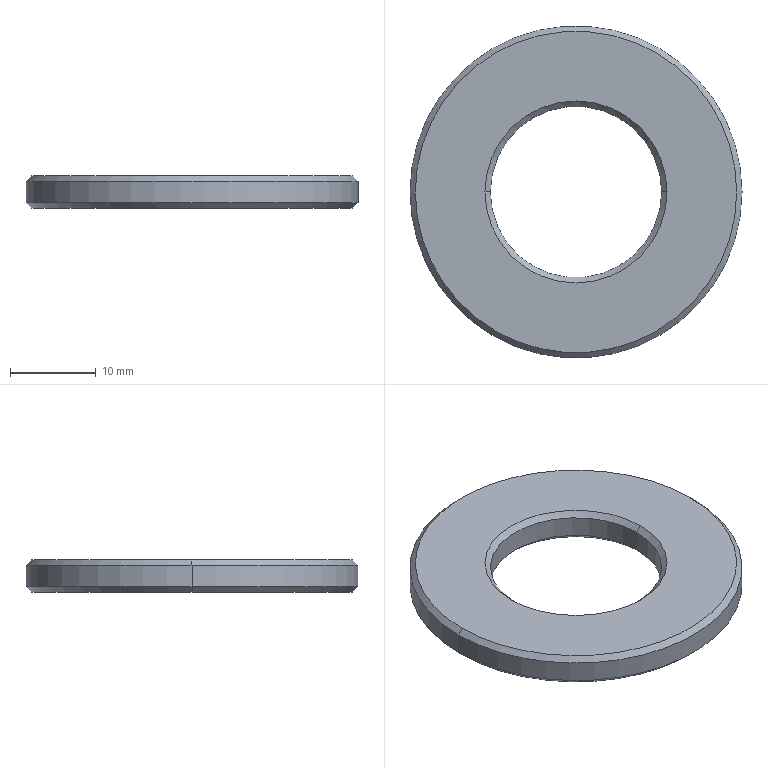Part | Creo | features DATUM PLANE 3, CHAMFER 1, COORDINATE SYSTEM 1, CURVE 1, PROTRUSION 1 | 1 solid | 14 faces | box 38.75 x 38.75 x 3.75 mm | volume 3172 mm3 | cone 8 | cylinder 4 | plane 2 | commonest cylinder face diameters 20 x2 38.75 x2
STEP:
#1=CARTESIAN_POINT('',(0.,0.,0.));
#2=DIRECTION('',(0.,0.,1.));
#3=DIRECTION('',(1.,0.,0.));
#4=AXIS2_PLACEMENT_3D('',#1,#2,#3);
#5=CARTESIAN_POINT('',(-18.75,0.,0.));
#6=VERTEX_POINT('',#5);
#7=CARTESIAN_POINT('',(18.75,0.,0.));
#8=VERTEX_POINT('',#7);
#9=CARTESIAN_POINT('',(0.,0.,0.));
#10=DIRECTION('',(0.,0.,-1.));
#11=DIRECTION('',(-1.,0.,0.));
#12=AXIS2_PLACEMENT_3D('',#9,#10,#11);
#13=CIRCLE('',#12,18.75);
#14=EDGE_CURVE('',#6,#8,#13,.T.);
#15=ORIENTED_EDGE('',*,*,#14,.F.);
#16=CARTESIAN_POINT('',(0.,0.,0.));
#17=DIRECTION('',(0.,0.,-1.));
#18=DIRECTION('',(1.,0.,0.));
#19=AXIS2_PLACEMENT_3D('',#16,#17,#18);
#20=CIRCLE('',#19,18.75);
#21=EDGE_CURVE('',#8,#6,#20,.T.);
#22=ORIENTED_EDGE('',*,*,#21,.F.);
#23=EDGE_LOOP('',(#15,#22));
#24=FACE_OUTER_BOUND('',#23,.F.);
#25=CARTESIAN_POINT('',(-10.625,0.,0.));
#26=VERTEX_POINT('',#25);
#27=CARTESIAN_POINT('',(10.625,0.,0.));
#28=VERTEX_POINT('',#27);
#29=CARTESIAN_POINT('',(0.,0.,0.));
#30=DIRECTION('',(0.,0.,1.));
#31=DIRECTION('',(-1.,0.,0.));
#32=AXIS2_PLACEMENT_3D('',#29,#30,#31);
#33=CIRCLE('',#32,10.625);
#34=EDGE_CURVE('',#26,#28,#33,.T.);
#35=ORIENTED_EDGE('',*,*,#34,.F.);
#36=CARTESIAN_POINT('',(0.,0.,0.));
#37=DIRECTION('',(0.,0.,1.));
#38=DIRECTION('',(1.,0.,0.));
#39=AXIS2_PLACEMENT_3D('',#36,#37,#38);
#40=CIRCLE('',#39,10.625);
#41=EDGE_CURVE('',#28,#26,#40,.T.);
#42=ORIENTED_EDGE('',*,*,#41,.F.);
#43=EDGE_LOOP('',(#35,#42));
#44=FACE_BOUND('',#43,.F.);
#45=CARTESIAN_POINT('',(0.,0.,0.));
#46=DIRECTION('',(0.,0.,1.));
#47=DIRECTION('',(1.,0.,0.));
#48=AXIS2_PLACEMENT_3D('',#45,#46,#47);
#49=PLANE('',#48);
#50=ADVANCED_FACE('',(#24,#44),#49,.F.);
#51=ORIENTED_EDGE('',*,*,#14,.T.);
#52=CARTESIAN_POINT('',(19.375,0.,0.625));
#53=VERTEX_POINT('',#52);
#54=CARTESIAN_POINT('',(18.75,0.000000003,0.));
#55=DIRECTION('',(0.7071,-0.000000001,0.7071));
#56=VECTOR('',#55,0.8839);
#57=LINE('',#54,#56);
#58=EDGE_CURVE('',#8,#53,#57,.T.);
#59=ORIENTED_EDGE('',*,*,#58,.T.);
#60=CARTESIAN_POINT('',(-19.375,0.,0.625));
#61=VERTEX_POINT('',#60);
#62=CARTESIAN_POINT('',(0.,0.,0.625));
#63=DIRECTION('',(0.,0.,-1.));
#64=DIRECTION('',(-1.,0.,0.));
#65=AXIS2_PLACEMENT_3D('',#62,#63,#64);
#66=CIRCLE('',#65,19.375);
#67=EDGE_CURVE('',#61,#53,#66,.T.);
#68=ORIENTED_EDGE('',*,*,#67,.F.);
#69=CARTESIAN_POINT('',(-18.75,-0.000000003,0.));
#70=DIRECTION('',(-0.7071,0.000000001,0.7071));
#71=VECTOR('',#70,0.8839);
#72=LINE('',#69,#71);
#73=EDGE_CURVE('',#6,#61,#72,.T.);
#74=ORIENTED_EDGE('',*,*,#73,.F.);
#75=EDGE_LOOP('',(#51,#59,#68,#74));
#76=FACE_OUTER_BOUND('',#75,.F.);
#77=CARTESIAN_POINT('',(0.,0.,0.3125));
#78=DIRECTION('',(0.,0.,1.));
#79=DIRECTION('',(0.,-1.,0.));
#80=AXIS2_PLACEMENT_3D('',#77,#78,#79);
#81=CONICAL_SURFACE('',#80,19.062,45.);
#82=ADVANCED_FACE('',(#76),#81,.T.);
#83=ORIENTED_EDGE('',*,*,#21,.T.);
#84=ORIENTED_EDGE('',*,*,#73,.T.);
#85=CARTESIAN_POINT('',(0.,0.,0.625));
#86=DIRECTION('',(0.,0.,-1.));
#87=DIRECTION('',(1.,0.,0.));
#88=AXIS2_PLACEMENT_3D('',#85,#86,#87);
#89=CIRCLE('',#88,19.375);
#90=EDGE_CURVE('',#53,#61,#89,.T.);
#91=ORIENTED_EDGE('',*,*,#90,.F.);
#92=ORIENTED_EDGE('',*,*,#58,.F.);
#93=EDGE_LOOP('',(#83,#84,#91,#92));
#94=FACE_OUTER_BOUND('',#93,.F.);
#95=CARTESIAN_POINT('',(0.,0.,0.3125));
#96=DIRECTION('',(0.,0.,1.));
#97=DIRECTION('',(0.,-1.,0.));
#98=AXIS2_PLACEMENT_3D('',#95,#96,#97);
#99=CONICAL_SURFACE('',#98,19.062,45.);
#100=ADVANCED_FACE('',(#94),#99,.T.);
#101=CARTESIAN_POINT('',(-19.375,0.,3.125));
#102=VERTEX_POINT('',#101);
#103=CARTESIAN_POINT('',(19.375,0.,3.125));
#104=VERTEX_POINT('',#103);
#105=CARTESIAN_POINT('',(0.,0.,3.125));
#106=DIRECTION('',(0.,0.,1.));
#107=DIRECTION('',(-1.,0.,0.));
#108=AXIS2_PLACEMENT_3D('',#105,#106,#107);
#109=CIRCLE('',#108,19.375);
#110=EDGE_CURVE('',#102,#104,#109,.T.);
#111=ORIENTED_EDGE('',*,*,#110,.T.);
#112=CARTESIAN_POINT('',(19.375,0.000000002,0.625));
#113=DIRECTION('',(0.,0.,1.));
#114=VECTOR('',#113,2.5);
#115=LINE('',#112,#114);
#116=EDGE_CURVE('',#53,#104,#115,.T.);
#117=ORIENTED_EDGE('',*,*,#116,.F.);
#118=ORIENTED_EDGE('',*,*,#90,.T.);
#119=CARTESIAN_POINT('',(-19.375,-0.000000002,0.625));
#120=DIRECTION('',(0.,0.,1.));
#121=VECTOR('',#120,2.5);
#122=LINE('',#119,#121);
#123=EDGE_CURVE('',#61,#102,#122,.T.);
#124=ORIENTED_EDGE('',*,*,#123,.T.);
#125=EDGE_LOOP('',(#111,#117,#118,#124));
#126=FACE_OUTER_BOUND('',#125,.F.);
#127=CARTESIAN_POINT('',(0.,0.,0.));
#128=DIRECTION('',(0.,0.,1.));
#129=DIRECTION('',(1.,0.,0.));
#130=AXIS2_PLACEMENT_3D('',#127,#128,#129);
#131=CYLINDRICAL_SURFACE('',#130,19.375);
#132=ADVANCED_FACE('',(#126),#131,.T.);
#133=CARTESIAN_POINT('',(-18.75,0.,3.75));
#134=VERTEX_POINT('',#133);
#135=CARTESIAN_POINT('',(18.75,0.,3.75));
#136=VERTEX_POINT('',#135);
#137=CARTESIAN_POINT('',(0.,0.,3.75));
#138=DIRECTION('',(0.,0.,1.));
#139=DIRECTION('',(-1.,0.,0.));
#140=AXIS2_PLACEMENT_3D('',#137,#138,#139);
#141=CIRCLE('',#140,18.75);
#142=EDGE_CURVE('',#134,#136,#141,.T.);
#143=ORIENTED_EDGE('',*,*,#142,.T.);
#144=CARTESIAN_POINT('',(18.75,0.000000003,3.75));
#145=DIRECTION('',(0.7071,-0.000000001,-0.7071));
#146=VECTOR('',#145,0.8839);
#147=LINE('',#144,#146);
#148=EDGE_CURVE('',#136,#104,#147,.T.);
#149=ORIENTED_EDGE('',*,*,#148,.T.);
#150=ORIENTED_EDGE('',*,*,#110,.F.);
#151=CARTESIAN_POINT('',(-18.75,-0.000000003,3.75));
#152=DIRECTION('',(-0.7071,0.000000001,-0.7071));
#153=VECTOR('',#152,0.8839);
#154=LINE('',#151,#153);
#155=EDGE_CURVE('',#134,#102,#154,.T.);
#156=ORIENTED_EDGE('',*,*,#155,.F.);
#157=EDGE_LOOP('',(#143,#149,#150,#156));
#158=FACE_OUTER_BOUND('',#157,.F.);
#159=CARTESIAN_POINT('',(0.,0.,3.438));
#160=DIRECTION('',(0.,0.,-1.));
#161=DIRECTION('',(0.,-1.,0.));
#162=AXIS2_PLACEMENT_3D('',#159,#160,#161);
#163=CONICAL_SURFACE('',#162,19.062,45.);
#164=ADVANCED_FACE('',(#158),#163,.T.);
#165=CARTESIAN_POINT('',(0.,0.,3.75));
#166=DIRECTION('',(0.,0.,1.));
#167=DIRECTION('',(1.,0.,0.));
#168=AXIS2_PLACEMENT_3D('',#165,#166,#167);
#169=CIRCLE('',#168,18.75);
#170=EDGE_CURVE('',#136,#134,#169,.T.);
#171=ORIENTED_EDGE('',*,*,#170,.F.);
#172=ORIENTED_EDGE('',*,*,#142,.F.);
#173=EDGE_LOOP('',(#171,#172));
#174=FACE_OUTER_BOUND('',#173,.F.);
#175=CARTESIAN_POINT('',(10.625,0.,3.75));
#176=VERTEX_POINT('',#175);
#177=CARTESIAN_POINT('',(-10.625,0.,3.75));
#178=VERTEX_POINT('',#177);
#179=CARTESIAN_POINT('',(0.,0.,3.75));
#180=DIRECTION('',(0.,0.,-1.));
#181=DIRECTION('',(1.,0.,0.));
#182=AXIS2_PLACEMENT_3D('',#179,#180,#181);
#183=CIRCLE('',#182,10.625);
#184=EDGE_CURVE('',#176,#178,#183,.T.);
#185=ORIENTED_EDGE('',*,*,#184,.F.);
#186=CARTESIAN_POINT('',(0.,0.,3.75));
#187=DIRECTION('',(0.,0.,-1.));
#188=DIRECTION('',(-1.,0.,0.));
#189=AXIS2_PLACEMENT_3D('',#186,#187,#188);
#190=CIRCLE('',#189,10.625);
#191=EDGE_CURVE('',#178,#176,#190,.T.);
#192=ORIENTED_EDGE('',*,*,#191,.F.);
#193=EDGE_LOOP('',(#185,#192));
#194=FACE_BOUND('',#193,.F.);
#195=CARTESIAN_POINT('',(0.,0.,3.75));
#196=DIRECTION('',(0.,0.,1.));
#197=DIRECTION('',(1.,0.,0.));
#198=AXIS2_PLACEMENT_3D('',#195,#196,#197);
#199=PLANE('',#198);
#200=ADVANCED_FACE('',(#174,#194),#199,.T.);
#201=ORIENTED_EDGE('',*,*,#170,.T.);
#202=ORIENTED_EDGE('',*,*,#155,.T.);
#203=CARTESIAN_POINT('',(0.,0.,3.125));
#204=DIRECTION('',(0.,0.,1.));
#205=DIRECTION('',(1.,0.,0.));
#206=AXIS2_PLACEMENT_3D('',#203,#204,#205);
#207=CIRCLE('',#206,19.375);
#208=EDGE_CURVE('',#104,#102,#207,.T.);
#209=ORIENTED_EDGE('',*,*,#208,.F.);
#210=ORIENTED_EDGE('',*,*,#148,.F.);
#211=EDGE_LOOP('',(#201,#202,#209,#210));
#212=FACE_OUTER_BOUND('',#211,.F.);
#213=CARTESIAN_POINT('',(0.,0.,3.438));
#214=DIRECTION('',(0.,0.,-1.));
#215=DIRECTION('',(0.,-1.,0.));
#216=AXIS2_PLACEMENT_3D('',#213,#214,#215);
#217=CONICAL_SURFACE('',#216,19.062,45.);
#218=ADVANCED_FACE('',(#212),#217,.T.);
#219=ORIENTED_EDGE('',*,*,#208,.T.);
#220=ORIENTED_EDGE('',*,*,#123,.F.);
#221=ORIENTED_EDGE('',*,*,#67,.T.);
#222=ORIENTED_EDGE('',*,*,#116,.T.);
#223=EDGE_LOOP('',(#219,#220,#221,#222));
#224=FACE_OUTER_BOUND('',#223,.F.);
#225=CARTESIAN_POINT('',(0.,0.,0.));
#226=DIRECTION('',(0.,0.,1.));
#227=DIRECTION('',(1.,0.,0.));
#228=AXIS2_PLACEMENT_3D('',#225,#226,#227);
#229=CYLINDRICAL_SURFACE('',#228,19.375);
#230=ADVANCED_FACE('',(#224),#229,.T.);
#231=ORIENTED_EDGE('',*,*,#184,.T.);
#232=CARTESIAN_POINT('',(-10.,0.,3.125));
#233=VERTEX_POINT('',#232);
#234=CARTESIAN_POINT('',(-10.625,-0.000000006,3.75));
#235=DIRECTION('',(0.7071,0.000000002,-0.7071));
#236=VECTOR('',#235,0.8839);
#237=LINE('',#234,#236);
#238=EDGE_CURVE('',#178,#233,#237,.T.);
#239=ORIENTED_EDGE('',*,*,#238,.T.);
#240=CARTESIAN_POINT('',(10.,0.,3.125));
#241=VERTEX_POINT('',#240);
#242=CARTESIAN_POINT('',(0.,0.,3.125));
#243=DIRECTION('',(0.,0.,-1.));
#244=DIRECTION('',(1.,0.,0.));
#245=AXIS2_PLACEMENT_3D('',#242,#243,#244);
#246=CIRCLE('',#245,10.);
#247=EDGE_CURVE('',#241,#233,#246,.T.);
#248=ORIENTED_EDGE('',*,*,#247,.F.);
#249=CARTESIAN_POINT('',(10.625,0.000000006,3.75));
#250=DIRECTION('',(-0.7071,-0.000000002,-0.7071));
#251=VECTOR('',#250,0.8839);
#252=LINE('',#249,#251);
#253=EDGE_CURVE('',#176,#241,#252,.T.);
#254=ORIENTED_EDGE('',*,*,#253,.F.);
#255=EDGE_LOOP('',(#231,#239,#248,#254));
#256=FACE_OUTER_BOUND('',#255,.F.);
#257=CARTESIAN_POINT('',(0.,0.,3.437));
#258=DIRECTION('',(0.,0.,1.));
#259=DIRECTION('',(0.,-1.,0.));
#260=AXIS2_PLACEMENT_3D('',#257,#258,#259);
#261=CONICAL_SURFACE('',#260,10.312,45.);
#262=ADVANCED_FACE('',(#256),#261,.F.);
#263=ORIENTED_EDGE('',*,*,#191,.T.);
#264=ORIENTED_EDGE('',*,*,#253,.T.);
#265=CARTESIAN_POINT('',(0.,0.,3.125));
#266=DIRECTION('',(0.,0.,-1.));
#267=DIRECTION('',(-1.,0.,0.));
#268=AXIS2_PLACEMENT_3D('',#265,#266,#267);
#269=CIRCLE('',#268,10.);
#270=EDGE_CURVE('',#233,#241,#269,.T.);
#271=ORIENTED_EDGE('',*,*,#270,.F.);
#272=ORIENTED_EDGE('',*,*,#238,.F.);
#273=EDGE_LOOP('',(#263,#264,#271,#272));
#274=FACE_OUTER_BOUND('',#273,.F.);
#275=CARTESIAN_POINT('',(0.,0.,3.437));
#276=DIRECTION('',(0.,0.,1.));
#277=DIRECTION('',(0.,-1.,0.));
#278=AXIS2_PLACEMENT_3D('',#275,#276,#277);
#279=CONICAL_SURFACE('',#278,10.312,45.);
#280=ADVANCED_FACE('',(#274),#279,.F.);
#281=CARTESIAN_POINT('',(10.,0.,0.625));
#282=VERTEX_POINT('',#281);
#283=CARTESIAN_POINT('',(-10.,0.,0.625));
#284=VERTEX_POINT('',#283);
#285=CARTESIAN_POINT('',(0.,0.,0.625));
#286=DIRECTION('',(0.,0.,1.));
#287=DIRECTION('',(1.,0.,0.));
#288=AXIS2_PLACEMENT_3D('',#285,#286,#287);
#289=CIRCLE('',#288,10.);
#290=EDGE_CURVE('',#282,#284,#289,.T.);
#291=ORIENTED_EDGE('',*,*,#290,.T.);
#292=CARTESIAN_POINT('',(-10.,-0.000000004,0.625));
#293=DIRECTION('',(0.,0.,1.));
#294=VECTOR('',#293,2.5);
#295=LINE('',#292,#294);
#296=EDGE_CURVE('',#284,#233,#295,.T.);
#297=ORIENTED_EDGE('',*,*,#296,.T.);
#298=ORIENTED_EDGE('',*,*,#270,.T.);
#299=CARTESIAN_POINT('',(10.,0.000000004,0.625));
#300=DIRECTION('',(0.,0.,1.));
#301=VECTOR('',#300,2.5);
#302=LINE('',#299,#301);
#303=EDGE_CURVE('',#282,#241,#302,.T.);
#304=ORIENTED_EDGE('',*,*,#303,.F.);
#305=EDGE_LOOP('',(#291,#297,#298,#304));
#306=FACE_OUTER_BOUND('',#305,.F.);
#307=CARTESIAN_POINT('',(0.,0.,0.));
#308=DIRECTION('',(0.,0.,1.));
#309=DIRECTION('',(1.,0.,0.));
#310=AXIS2_PLACEMENT_3D('',#307,#308,#309);
#311=CYLINDRICAL_SURFACE('',#310,10.);
#312=ADVANCED_FACE('',(#306),#311,.F.);
#313=ORIENTED_EDGE('',*,*,#41,.T.);
#314=CARTESIAN_POINT('',(-10.625,-0.000000006,0.));
#315=DIRECTION('',(0.7071,0.000000002,0.7071));
#316=VECTOR('',#315,0.8839);
#317=LINE('',#314,#316);
#318=EDGE_CURVE('',#26,#284,#317,.T.);
#319=ORIENTED_EDGE('',*,*,#318,.T.);
#320=ORIENTED_EDGE('',*,*,#290,.F.);
#321=CARTESIAN_POINT('',(10.625,0.000000006,0.));
#322=DIRECTION('',(-0.7071,-0.000000002,0.7071));
#323=VECTOR('',#322,0.8839);
#324=LINE('',#321,#323);
#325=EDGE_CURVE('',#28,#282,#324,.T.);
#326=ORIENTED_EDGE('',*,*,#325,.F.);
#327=EDGE_LOOP('',(#313,#319,#320,#326));
#328=FACE_OUTER_BOUND('',#327,.F.);
#329=CARTESIAN_POINT('',(0.,0.,0.3125));
#330=DIRECTION('',(0.,0.,-1.));
#331=DIRECTION('',(0.,-1.,0.));
#332=AXIS2_PLACEMENT_3D('',#329,#330,#331);
#333=CONICAL_SURFACE('',#332,10.312,45.);
#334=ADVANCED_FACE('',(#328),#333,.F.);
#335=ORIENTED_EDGE('',*,*,#34,.T.);
#336=ORIENTED_EDGE('',*,*,#325,.T.);
#337=CARTESIAN_POINT('',(0.,0.,0.625));
#338=DIRECTION('',(0.,0.,1.));
#339=DIRECTION('',(-1.,0.,0.));
#340=AXIS2_PLACEMENT_3D('',#337,#338,#339);
#341=CIRCLE('',#340,10.);
#342=EDGE_CURVE('',#284,#282,#341,.T.);
#343=ORIENTED_EDGE('',*,*,#342,.F.);
#344=ORIENTED_EDGE('',*,*,#318,.F.);
#345=EDGE_LOOP('',(#335,#336,#343,#344));
#346=FACE_OUTER_BOUND('',#345,.F.);
#347=CARTESIAN_POINT('',(0.,0.,0.3125));
#348=DIRECTION('',(0.,0.,-1.));
#349=DIRECTION('',(0.,-1.,0.));
#350=AXIS2_PLACEMENT_3D('',#347,#348,#349);
#351=CONICAL_SURFACE('',#350,10.312,45.);
#352=ADVANCED_FACE('',(#346),#351,.F.);
#353=ORIENTED_EDGE('',*,*,#342,.T.);
#354=ORIENTED_EDGE('',*,*,#303,.T.);
#355=ORIENTED_EDGE('',*,*,#247,.T.);
#356=ORIENTED_EDGE('',*,*,#296,.F.);
#357=EDGE_LOOP('',(#353,#354,#355,#356));
#358=FACE_OUTER_BOUND('',#357,.F.);
#359=CARTESIAN_POINT('',(0.,0.,0.));
#360=DIRECTION('',(0.,0.,1.));
#361=DIRECTION('',(1.,0.,0.));
#362=AXIS2_PLACEMENT_3D('',#359,#360,#361);
#363=CYLINDRICAL_SURFACE('',#362,10.);
#364=ADVANCED_FACE('',(#358),#363,.F.);
#365=CLOSED_SHELL('',(#50,#82,#100,#132,#164,#200,#218,#230,#262,#280,#312,#334,#352,#364));
#366=MANIFOLD_SOLID_BREP('',#365);
#367=(LENGTH_UNIT()NAMED_UNIT(*)SI_UNIT(.MILLI.,.METRE.));
#368=UNCERTAINTY_MEASURE_WITH_UNIT(LENGTH_MEASURE(0.005495),#367,'','');
#369=(NAMED_UNIT(*)PLANE_ANGLE_UNIT()SI_UNIT($,.RADIAN.));
#370=PLANE_ANGLE_MEASURE_WITH_UNIT(PLANE_ANGLE_MEASURE(0.01745),#369);
#371=(CONVERSION_BASED_UNIT('DEGREE',#370)NAMED_UNIT(*)PLANE_ANGLE_UNIT());
#372=(NAMED_UNIT(*)SI_UNIT($,.STERADIAN.)SOLID_ANGLE_UNIT());
#373=(GEOMETRIC_REPRESENTATION_CONTEXT(3)GLOBAL_UNCERTAINTY_ASSIGNED_CONTEXT((#368))GLOBAL_UNIT_ASSIGNED_CONTEXT((#367,#371,#372))REPRESENTATION_CONTEXT('',''));
#374=ADVANCED_BREP_SHAPE_REPRESENTATION('',(#4,#366),#373);